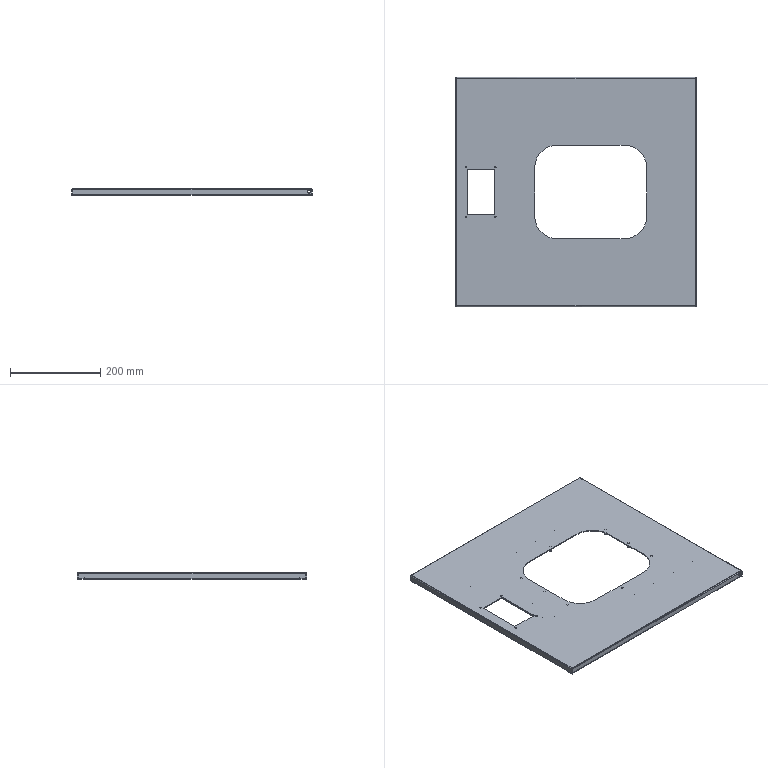Part | STEP file | 4 solids | 238 faces | box 533 x 508 x 15 mm | volume 546675 mm3 | plane 142 | cylinder 84 | spline 12 | commonest cylinder face diameters 5 x40 1 x14 3.3 x8 4.6 x8 3.4 x6 7 x4